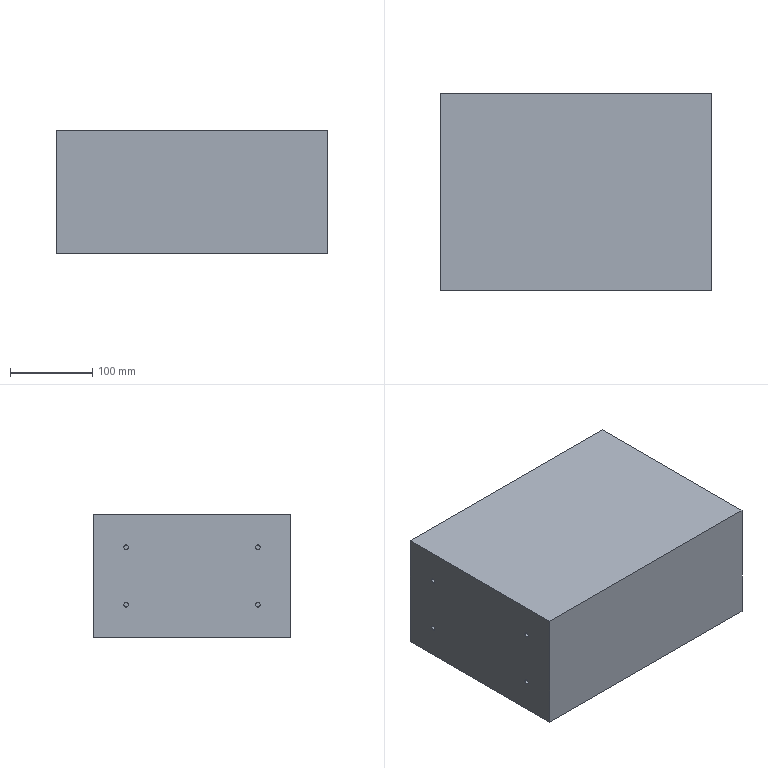Part | SolidWorks | features Cut 2, Extrusion 1 | 1 solid | 24 faces | box 330 x 240 x 150 mm | volume 11869232 mm3 | cylinder 12 | plane 12 | commonest cylinder face diameters 5.5 x8 25 x4
STEP:
#1=CARTESIAN_POINT('',(-155.,-77.25,40.));
#2=VERTEX_POINT('',#1);
#3=CARTESIAN_POINT('',(-155.,-82.75,40.));
#4=VERTEX_POINT('',#3);
#5=CARTESIAN_POINT('',(-155.,-80.,40.));
#6=DIRECTION('',(-1.,0.,0.));
#7=DIRECTION('',(0.,-1.,0.));
#8=AXIS2_PLACEMENT_3D('',#5,#6,#7);
#9=CIRCLE('',#8,2.75);
#10=EDGE_CURVE('',#2,#4,#9,.T.);
#11=ORIENTED_EDGE('',*,*,#10,.F.);
#12=CARTESIAN_POINT('',(-165.,-77.25,40.));
#13=VERTEX_POINT('',#12);
#14=CARTESIAN_POINT('',(-155.,-77.25,40.));
#15=DIRECTION('',(-1.,0.,0.));
#16=VECTOR('',#15,1000.);
#17=LINE('',#14,#16);
#18=EDGE_CURVE('',#2,#13,#17,.T.);
#19=ORIENTED_EDGE('',*,*,#18,.T.);
#20=CARTESIAN_POINT('',(-165.,-82.75,40.));
#21=VERTEX_POINT('',#20);
#22=CARTESIAN_POINT('',(-165.,-80.,40.));
#23=DIRECTION('',(-1.,0.,0.));
#24=DIRECTION('',(0.,-1.,0.));
#25=AXIS2_PLACEMENT_3D('',#22,#23,#24);
#26=CIRCLE('',#25,2.75);
#27=EDGE_CURVE('',#13,#21,#26,.T.);
#28=ORIENTED_EDGE('',*,*,#27,.T.);
#29=CARTESIAN_POINT('',(-155.,-82.75,40.));
#30=DIRECTION('',(-1.,0.,0.));
#31=VECTOR('',#30,1000.);
#32=LINE('',#29,#31);
#33=EDGE_CURVE('',#4,#21,#32,.T.);
#34=ORIENTED_EDGE('',*,*,#33,.F.);
#35=EDGE_LOOP('',(#11,#19,#28,#34));
#36=FACE_OUTER_BOUND('',#35,.T.);
#37=CARTESIAN_POINT('',(-155.,-80.,40.));
#38=DIRECTION('',(-1.,0.,0.));
#39=DIRECTION('',(0.,-1.,0.));
#40=AXIS2_PLACEMENT_3D('',#37,#38,#39);
#41=CYLINDRICAL_SURFACE('',#40,2.75);
#42=ADVANCED_FACE('',(#36),#41,.F.);
#43=CARTESIAN_POINT('',(-155.,-77.25,110.));
#44=VERTEX_POINT('',#43);
#45=CARTESIAN_POINT('',(-155.,-82.75,110.));
#46=VERTEX_POINT('',#45);
#47=CARTESIAN_POINT('',(-155.,-80.,110.));
#48=DIRECTION('',(-1.,0.,0.));
#49=DIRECTION('',(0.,-1.,0.));
#50=AXIS2_PLACEMENT_3D('',#47,#48,#49);
#51=CIRCLE('',#50,2.75);
#52=EDGE_CURVE('',#44,#46,#51,.T.);
#53=ORIENTED_EDGE('',*,*,#52,.F.);
#54=CARTESIAN_POINT('',(-165.,-77.25,110.));
#55=VERTEX_POINT('',#54);
#56=CARTESIAN_POINT('',(-155.,-77.25,110.));
#57=DIRECTION('',(-1.,0.,0.));
#58=VECTOR('',#57,1000.);
#59=LINE('',#56,#58);
#60=EDGE_CURVE('',#44,#55,#59,.T.);
#61=ORIENTED_EDGE('',*,*,#60,.T.);
#62=CARTESIAN_POINT('',(-165.,-82.75,110.));
#63=VERTEX_POINT('',#62);
#64=CARTESIAN_POINT('',(-165.,-80.,110.));
#65=DIRECTION('',(-1.,0.,0.));
#66=DIRECTION('',(0.,-1.,0.));
#67=AXIS2_PLACEMENT_3D('',#64,#65,#66);
#68=CIRCLE('',#67,2.75);
#69=EDGE_CURVE('',#55,#63,#68,.T.);
#70=ORIENTED_EDGE('',*,*,#69,.T.);
#71=CARTESIAN_POINT('',(-155.,-82.75,110.));
#72=DIRECTION('',(-1.,0.,0.));
#73=VECTOR('',#72,1000.);
#74=LINE('',#71,#73);
#75=EDGE_CURVE('',#46,#63,#74,.T.);
#76=ORIENTED_EDGE('',*,*,#75,.F.);
#77=EDGE_LOOP('',(#53,#61,#70,#76));
#78=FACE_OUTER_BOUND('',#77,.T.);
#79=CARTESIAN_POINT('',(-155.,-80.,110.));
#80=DIRECTION('',(-1.,0.,0.));
#81=DIRECTION('',(0.,-1.,0.));
#82=AXIS2_PLACEMENT_3D('',#79,#80,#81);
#83=CYLINDRICAL_SURFACE('',#82,2.75);
#84=ADVANCED_FACE('',(#78),#83,.F.);
#85=CARTESIAN_POINT('',(-155.,82.75,110.));
#86=VERTEX_POINT('',#85);
#87=CARTESIAN_POINT('',(-155.,77.25,110.));
#88=VERTEX_POINT('',#87);
#89=CARTESIAN_POINT('',(-155.,80.,110.));
#90=DIRECTION('',(-1.,0.,0.));
#91=DIRECTION('',(0.,-1.,0.));
#92=AXIS2_PLACEMENT_3D('',#89,#90,#91);
#93=CIRCLE('',#92,2.75);
#94=EDGE_CURVE('',#86,#88,#93,.T.);
#95=ORIENTED_EDGE('',*,*,#94,.F.);
#96=CARTESIAN_POINT('',(-165.,82.75,110.));
#97=VERTEX_POINT('',#96);
#98=CARTESIAN_POINT('',(-155.,82.75,110.));
#99=DIRECTION('',(-1.,0.,0.));
#100=VECTOR('',#99,1000.);
#101=LINE('',#98,#100);
#102=EDGE_CURVE('',#86,#97,#101,.T.);
#103=ORIENTED_EDGE('',*,*,#102,.T.);
#104=CARTESIAN_POINT('',(-165.,77.25,110.));
#105=VERTEX_POINT('',#104);
#106=CARTESIAN_POINT('',(-165.,80.,110.));
#107=DIRECTION('',(-1.,0.,0.));
#108=DIRECTION('',(0.,-1.,0.));
#109=AXIS2_PLACEMENT_3D('',#106,#107,#108);
#110=CIRCLE('',#109,2.75);
#111=EDGE_CURVE('',#97,#105,#110,.T.);
#112=ORIENTED_EDGE('',*,*,#111,.T.);
#113=CARTESIAN_POINT('',(-155.,77.25,110.));
#114=DIRECTION('',(-1.,0.,0.));
#115=VECTOR('',#114,1000.);
#116=LINE('',#113,#115);
#117=EDGE_CURVE('',#88,#105,#116,.T.);
#118=ORIENTED_EDGE('',*,*,#117,.F.);
#119=EDGE_LOOP('',(#95,#103,#112,#118));
#120=FACE_OUTER_BOUND('',#119,.T.);
#121=CARTESIAN_POINT('',(-155.,80.,110.));
#122=DIRECTION('',(-1.,0.,0.));
#123=DIRECTION('',(0.,-1.,0.));
#124=AXIS2_PLACEMENT_3D('',#121,#122,#123);
#125=CYLINDRICAL_SURFACE('',#124,2.75);
#126=ADVANCED_FACE('',(#120),#125,.F.);
#127=CARTESIAN_POINT('',(-155.,82.75,40.));
#128=VERTEX_POINT('',#127);
#129=CARTESIAN_POINT('',(-155.,77.25,40.));
#130=VERTEX_POINT('',#129);
#131=CARTESIAN_POINT('',(-155.,80.,40.));
#132=DIRECTION('',(-1.,0.,0.));
#133=DIRECTION('',(0.,-1.,0.));
#134=AXIS2_PLACEMENT_3D('',#131,#132,#133);
#135=CIRCLE('',#134,2.75);
#136=EDGE_CURVE('',#128,#130,#135,.T.);
#137=ORIENTED_EDGE('',*,*,#136,.F.);
#138=CARTESIAN_POINT('',(-165.,82.75,40.));
#139=VERTEX_POINT('',#138);
#140=CARTESIAN_POINT('',(-155.,82.75,40.));
#141=DIRECTION('',(-1.,0.,0.));
#142=VECTOR('',#141,1000.);
#143=LINE('',#140,#142);
#144=EDGE_CURVE('',#128,#139,#143,.T.);
#145=ORIENTED_EDGE('',*,*,#144,.T.);
#146=CARTESIAN_POINT('',(-165.,77.25,40.));
#147=VERTEX_POINT('',#146);
#148=CARTESIAN_POINT('',(-165.,80.,40.));
#149=DIRECTION('',(-1.,0.,0.));
#150=DIRECTION('',(0.,-1.,0.));
#151=AXIS2_PLACEMENT_3D('',#148,#149,#150);
#152=CIRCLE('',#151,2.75);
#153=EDGE_CURVE('',#139,#147,#152,.T.);
#154=ORIENTED_EDGE('',*,*,#153,.T.);
#155=CARTESIAN_POINT('',(-155.,77.25,40.));
#156=DIRECTION('',(-1.,0.,0.));
#157=VECTOR('',#156,1000.);
#158=LINE('',#155,#157);
#159=EDGE_CURVE('',#130,#147,#158,.T.);
#160=ORIENTED_EDGE('',*,*,#159,.F.);
#161=EDGE_LOOP('',(#137,#145,#154,#160));
#162=FACE_OUTER_BOUND('',#161,.T.);
#163=CARTESIAN_POINT('',(-155.,80.,40.));
#164=DIRECTION('',(-1.,0.,0.));
#165=DIRECTION('',(0.,-1.,0.));
#166=AXIS2_PLACEMENT_3D('',#163,#164,#165);
#167=CYLINDRICAL_SURFACE('',#166,2.75);
#168=ADVANCED_FACE('',(#162),#167,.F.);
#169=CARTESIAN_POINT('',(155.,-72.5,75.));
#170=VERTEX_POINT('',#169);
#171=CARTESIAN_POINT('',(155.,-47.5,75.));
#172=VERTEX_POINT('',#171);
#173=CARTESIAN_POINT('',(155.,-60.,75.));
#174=DIRECTION('',(1.,0.,0.));
#175=DIRECTION('',(0.,1.,0.));
#176=AXIS2_PLACEMENT_3D('',#173,#174,#175);
#177=CIRCLE('',#176,12.5);
#178=EDGE_CURVE('',#170,#172,#177,.T.);
#179=ORIENTED_EDGE('',*,*,#178,.F.);
#180=CARTESIAN_POINT('',(165.,-72.5,75.));
#181=VERTEX_POINT('',#180);
#182=CARTESIAN_POINT('',(155.,-72.5,75.));
#183=DIRECTION('',(1.,0.,0.));
#184=VECTOR('',#183,1000.);
#185=LINE('',#182,#184);
#186=EDGE_CURVE('',#170,#181,#185,.T.);
#187=ORIENTED_EDGE('',*,*,#186,.T.);
#188=CARTESIAN_POINT('',(165.,-47.5,75.));
#189=VERTEX_POINT('',#188);
#190=CARTESIAN_POINT('',(165.,-60.,75.));
#191=DIRECTION('',(1.,0.,0.));
#192=DIRECTION('',(0.,1.,0.));
#193=AXIS2_PLACEMENT_3D('',#190,#191,#192);
#194=CIRCLE('',#193,12.5);
#195=EDGE_CURVE('',#181,#189,#194,.T.);
#196=ORIENTED_EDGE('',*,*,#195,.T.);
#197=CARTESIAN_POINT('',(155.,-47.5,75.));
#198=DIRECTION('',(1.,0.,0.));
#199=VECTOR('',#198,1000.);
#200=LINE('',#197,#199);
#201=EDGE_CURVE('',#172,#189,#200,.T.);
#202=ORIENTED_EDGE('',*,*,#201,.F.);
#203=EDGE_LOOP('',(#179,#187,#196,#202));
#204=FACE_OUTER_BOUND('',#203,.T.);
#205=CARTESIAN_POINT('',(155.,-60.,75.));
#206=DIRECTION('',(1.,0.,0.));
#207=DIRECTION('',(0.,1.,0.));
#208=AXIS2_PLACEMENT_3D('',#205,#206,#207);
#209=CYLINDRICAL_SURFACE('',#208,12.5);
#210=ADVANCED_FACE('',(#204),#209,.F.);
#211=CARTESIAN_POINT('',(155.,47.5,75.));
#212=VERTEX_POINT('',#211);
#213=CARTESIAN_POINT('',(155.,72.5,75.));
#214=VERTEX_POINT('',#213);
#215=CARTESIAN_POINT('',(155.,60.,75.));
#216=DIRECTION('',(1.,0.,0.));
#217=DIRECTION('',(0.,1.,0.));
#218=AXIS2_PLACEMENT_3D('',#215,#216,#217);
#219=CIRCLE('',#218,12.5);
#220=EDGE_CURVE('',#212,#214,#219,.T.);
#221=ORIENTED_EDGE('',*,*,#220,.F.);
#222=CARTESIAN_POINT('',(165.,47.5,75.));
#223=VERTEX_POINT('',#222);
#224=CARTESIAN_POINT('',(155.,47.5,75.));
#225=DIRECTION('',(1.,0.,0.));
#226=VECTOR('',#225,1000.);
#227=LINE('',#224,#226);
#228=EDGE_CURVE('',#212,#223,#227,.T.);
#229=ORIENTED_EDGE('',*,*,#228,.T.);
#230=CARTESIAN_POINT('',(165.,72.5,75.));
#231=VERTEX_POINT('',#230);
#232=CARTESIAN_POINT('',(165.,60.,75.));
#233=DIRECTION('',(1.,0.,0.));
#234=DIRECTION('',(0.,1.,0.));
#235=AXIS2_PLACEMENT_3D('',#232,#233,#234);
#236=CIRCLE('',#235,12.5);
#237=EDGE_CURVE('',#223,#231,#236,.T.);
#238=ORIENTED_EDGE('',*,*,#237,.T.);
#239=CARTESIAN_POINT('',(155.,72.5,75.));
#240=DIRECTION('',(1.,0.,0.));
#241=VECTOR('',#240,1000.);
#242=LINE('',#239,#241);
#243=EDGE_CURVE('',#214,#231,#242,.T.);
#244=ORIENTED_EDGE('',*,*,#243,.F.);
#245=EDGE_LOOP('',(#221,#229,#238,#244));
#246=FACE_OUTER_BOUND('',#245,.T.);
#247=CARTESIAN_POINT('',(155.,60.,75.));
#248=DIRECTION('',(1.,0.,0.));
#249=DIRECTION('',(0.,1.,0.));
#250=AXIS2_PLACEMENT_3D('',#247,#248,#249);
#251=CYLINDRICAL_SURFACE('',#250,12.5);
#252=ADVANCED_FACE('',(#246),#251,.F.);
#253=CARTESIAN_POINT('',(165.,-60.,75.));
#254=DIRECTION('',(1.,0.,0.));
#255=DIRECTION('',(0.,1.,0.));
#256=AXIS2_PLACEMENT_3D('',#253,#254,#255);
#257=CIRCLE('',#256,12.5);
#258=EDGE_CURVE('',#189,#181,#257,.T.);
#259=ORIENTED_EDGE('',*,*,#258,.F.);
#260=ORIENTED_EDGE('',*,*,#195,.F.);
#261=EDGE_LOOP('',(#259,#260));
#262=FACE_BOUND('',#261,.T.);
#263=CARTESIAN_POINT('',(165.,60.,75.));
#264=DIRECTION('',(1.,0.,0.));
#265=DIRECTION('',(0.,1.,0.));
#266=AXIS2_PLACEMENT_3D('',#263,#264,#265);
#267=CIRCLE('',#266,12.5);
#268=EDGE_CURVE('',#231,#223,#267,.T.);
#269=ORIENTED_EDGE('',*,*,#268,.F.);
#270=ORIENTED_EDGE('',*,*,#237,.F.);
#271=EDGE_LOOP('',(#269,#270));
#272=FACE_BOUND('',#271,.T.);
#273=CARTESIAN_POINT('',(165.,-120.,0.));
#274=VERTEX_POINT('',#273);
#275=CARTESIAN_POINT('',(165.,120.,0.));
#276=VERTEX_POINT('',#275);
#277=CARTESIAN_POINT('',(165.,120.,0.));
#278=DIRECTION('',(0.,1.,0.));
#279=VECTOR('',#278,1000.);
#280=LINE('',#277,#279);
#281=EDGE_CURVE('',#274,#276,#280,.T.);
#282=ORIENTED_EDGE('',*,*,#281,.T.);
#283=CARTESIAN_POINT('',(165.,120.,150.));
#284=VERTEX_POINT('',#283);
#285=CARTESIAN_POINT('',(165.,120.,150.));
#286=DIRECTION('',(0.,0.,-1.));
#287=VECTOR('',#286,1000.);
#288=LINE('',#285,#287);
#289=EDGE_CURVE('',#284,#276,#288,.T.);
#290=ORIENTED_EDGE('',*,*,#289,.F.);
#291=CARTESIAN_POINT('',(165.,-120.,150.));
#292=VERTEX_POINT('',#291);
#293=CARTESIAN_POINT('',(165.,120.,150.));
#294=DIRECTION('',(0.,1.,0.));
#295=VECTOR('',#294,1000.);
#296=LINE('',#293,#295);
#297=EDGE_CURVE('',#292,#284,#296,.T.);
#298=ORIENTED_EDGE('',*,*,#297,.F.);
#299=CARTESIAN_POINT('',(165.,-120.,150.));
#300=DIRECTION('',(0.,0.,-1.));
#301=VECTOR('',#300,1000.);
#302=LINE('',#299,#301);
#303=EDGE_CURVE('',#292,#274,#302,.T.);
#304=ORIENTED_EDGE('',*,*,#303,.T.);
#305=EDGE_LOOP('',(#282,#290,#298,#304));
#306=FACE_OUTER_BOUND('',#305,.T.);
#307=CARTESIAN_POINT('',(165.,120.,150.));
#308=DIRECTION('',(-1.,0.,0.));
#309=DIRECTION('',(0.,-1.,0.));
#310=AXIS2_PLACEMENT_3D('',#307,#308,#309);
#311=PLANE('',#310);
#312=ADVANCED_FACE('',(#262,#272,#306),#311,.F.);
#313=CARTESIAN_POINT('',(-165.,120.,0.));
#314=VERTEX_POINT('',#313);
#315=CARTESIAN_POINT('',(-165.,120.,0.));
#316=DIRECTION('',(-1.,0.,0.));
#317=VECTOR('',#316,1000.);
#318=LINE('',#315,#317);
#319=EDGE_CURVE('',#276,#314,#318,.T.);
#320=ORIENTED_EDGE('',*,*,#319,.T.);
#321=CARTESIAN_POINT('',(-165.,120.,150.));
#322=VERTEX_POINT('',#321);
#323=CARTESIAN_POINT('',(-165.,120.,150.));
#324=DIRECTION('',(0.,0.,-1.));
#325=VECTOR('',#324,1000.);
#326=LINE('',#323,#325);
#327=EDGE_CURVE('',#322,#314,#326,.T.);
#328=ORIENTED_EDGE('',*,*,#327,.F.);
#329=CARTESIAN_POINT('',(-165.,120.,150.));
#330=DIRECTION('',(-1.,0.,0.));
#331=VECTOR('',#330,1000.);
#332=LINE('',#329,#331);
#333=EDGE_CURVE('',#284,#322,#332,.T.);
#334=ORIENTED_EDGE('',*,*,#333,.F.);
#335=ORIENTED_EDGE('',*,*,#289,.T.);
#336=EDGE_LOOP('',(#320,#328,#334,#335));
#337=FACE_OUTER_BOUND('',#336,.T.);
#338=CARTESIAN_POINT('',(-165.,120.,150.));
#339=DIRECTION('',(0.,-1.,0.));
#340=DIRECTION('',(0.,0.,-1.));
#341=AXIS2_PLACEMENT_3D('',#338,#339,#340);
#342=PLANE('',#341);
#343=ADVANCED_FACE('',(#337),#342,.F.);
#344=CARTESIAN_POINT('',(-165.,-80.,40.));
#345=DIRECTION('',(-1.,0.,0.));
#346=DIRECTION('',(0.,-1.,0.));
#347=AXIS2_PLACEMENT_3D('',#344,#345,#346);
#348=CIRCLE('',#347,2.75);
#349=EDGE_CURVE('',#21,#13,#348,.T.);
#350=ORIENTED_EDGE('',*,*,#349,.F.);
#351=ORIENTED_EDGE('',*,*,#27,.F.);
#352=EDGE_LOOP('',(#350,#351));
#353=FACE_BOUND('',#352,.T.);
#354=CARTESIAN_POINT('',(-165.,-80.,110.));
#355=DIRECTION('',(-1.,0.,0.));
#356=DIRECTION('',(0.,-1.,0.));
#357=AXIS2_PLACEMENT_3D('',#354,#355,#356);
#358=CIRCLE('',#357,2.75);
#359=EDGE_CURVE('',#63,#55,#358,.T.);
#360=ORIENTED_EDGE('',*,*,#359,.F.);
#361=ORIENTED_EDGE('',*,*,#69,.F.);
#362=EDGE_LOOP('',(#360,#361));
#363=FACE_BOUND('',#362,.T.);
#364=CARTESIAN_POINT('',(-165.,80.,110.));
#365=DIRECTION('',(-1.,0.,0.));
#366=DIRECTION('',(0.,-1.,0.));
#367=AXIS2_PLACEMENT_3D('',#364,#365,#366);
#368=CIRCLE('',#367,2.75);
#369=EDGE_CURVE('',#105,#97,#368,.T.);
#370=ORIENTED_EDGE('',*,*,#369,.F.);
#371=ORIENTED_EDGE('',*,*,#111,.F.);
#372=EDGE_LOOP('',(#370,#371));
#373=FACE_BOUND('',#372,.T.);
#374=CARTESIAN_POINT('',(-165.,80.,40.));
#375=DIRECTION('',(-1.,0.,0.));
#376=DIRECTION('',(0.,-1.,0.));
#377=AXIS2_PLACEMENT_3D('',#374,#375,#376);
#378=CIRCLE('',#377,2.75);
#379=EDGE_CURVE('',#147,#139,#378,.T.);
#380=ORIENTED_EDGE('',*,*,#379,.F.);
#381=ORIENTED_EDGE('',*,*,#153,.F.);
#382=EDGE_LOOP('',(#380,#381));
#383=FACE_BOUND('',#382,.T.);
#384=CARTESIAN_POINT('',(-165.,-120.,0.));
#385=VERTEX_POINT('',#384);
#386=CARTESIAN_POINT('',(-165.,120.,0.));
#387=DIRECTION('',(0.,-1.,0.));
#388=VECTOR('',#387,1000.);
#389=LINE('',#386,#388);
#390=EDGE_CURVE('',#314,#385,#389,.T.);
#391=ORIENTED_EDGE('',*,*,#390,.T.);
#392=CARTESIAN_POINT('',(-165.,-120.,150.));
#393=VERTEX_POINT('',#392);
#394=CARTESIAN_POINT('',(-165.,-120.,150.));
#395=DIRECTION('',(0.,0.,-1.));
#396=VECTOR('',#395,1000.);
#397=LINE('',#394,#396);
#398=EDGE_CURVE('',#393,#385,#397,.T.);
#399=ORIENTED_EDGE('',*,*,#398,.F.);
#400=CARTESIAN_POINT('',(-165.,120.,150.));
#401=DIRECTION('',(0.,-1.,0.));
#402=VECTOR('',#401,1000.);
#403=LINE('',#400,#402);
#404=EDGE_CURVE('',#322,#393,#403,.T.);
#405=ORIENTED_EDGE('',*,*,#404,.F.);
#406=ORIENTED_EDGE('',*,*,#327,.T.);
#407=EDGE_LOOP('',(#391,#399,#405,#406));
#408=FACE_OUTER_BOUND('',#407,.T.);
#409=CARTESIAN_POINT('',(-165.,120.,150.));
#410=DIRECTION('',(1.,0.,0.));
#411=DIRECTION('',(0.,0.,-1.));
#412=AXIS2_PLACEMENT_3D('',#409,#410,#411);
#413=PLANE('',#412);
#414=ADVANCED_FACE('',(#353,#363,#373,#383,#408),#413,.F.);
#415=CARTESIAN_POINT('',(-165.,-120.,0.));
#416=DIRECTION('',(1.,0.,0.));
#417=VECTOR('',#416,1000.);
#418=LINE('',#415,#417);
#419=EDGE_CURVE('',#385,#274,#418,.T.);
#420=ORIENTED_EDGE('',*,*,#419,.T.);
#421=ORIENTED_EDGE('',*,*,#303,.F.);
#422=CARTESIAN_POINT('',(-165.,-120.,150.));
#423=DIRECTION('',(1.,0.,0.));
#424=VECTOR('',#423,1000.);
#425=LINE('',#422,#424);
#426=EDGE_CURVE('',#393,#292,#425,.T.);
#427=ORIENTED_EDGE('',*,*,#426,.F.);
#428=ORIENTED_EDGE('',*,*,#398,.T.);
#429=EDGE_LOOP('',(#420,#421,#427,#428));
#430=FACE_OUTER_BOUND('',#429,.T.);
#431=CARTESIAN_POINT('',(-165.,-120.,150.));
#432=DIRECTION('',(0.,1.,0.));
#433=DIRECTION('',(0.,0.,1.));
#434=AXIS2_PLACEMENT_3D('',#431,#432,#433);
#435=PLANE('',#434);
#436=ADVANCED_FACE('',(#430),#435,.F.);
#437=ORIENTED_EDGE('',*,*,#297,.T.);
#438=ORIENTED_EDGE('',*,*,#333,.T.);
#439=ORIENTED_EDGE('',*,*,#404,.T.);
#440=ORIENTED_EDGE('',*,*,#426,.T.);
#441=EDGE_LOOP('',(#437,#438,#439,#440));
#442=FACE_OUTER_BOUND('',#441,.T.);
#443=CARTESIAN_POINT('',(0.,0.,150.));
#444=DIRECTION('',(0.,0.,1.));
#445=DIRECTION('',(1.,0.,0.));
#446=AXIS2_PLACEMENT_3D('',#443,#444,#445);
#447=PLANE('',#446);
#448=ADVANCED_FACE('',(#442),#447,.T.);
#449=ORIENTED_EDGE('',*,*,#281,.F.);
#450=ORIENTED_EDGE('',*,*,#419,.F.);
#451=ORIENTED_EDGE('',*,*,#390,.F.);
#452=ORIENTED_EDGE('',*,*,#319,.F.);
#453=EDGE_LOOP('',(#449,#450,#451,#452));
#454=FACE_OUTER_BOUND('',#453,.T.);
#455=CARTESIAN_POINT('',(0.,0.,0.));
#456=DIRECTION('',(0.,0.,1.));
#457=DIRECTION('',(1.,0.,0.));
#458=AXIS2_PLACEMENT_3D('',#455,#456,#457);
#459=PLANE('',#458);
#460=ADVANCED_FACE('',(#454),#459,.F.);
#461=ORIENTED_EDGE('',*,*,#228,.F.);
#462=CARTESIAN_POINT('',(155.,60.,75.));
#463=DIRECTION('',(1.,0.,0.));
#464=DIRECTION('',(0.,1.,0.));
#465=AXIS2_PLACEMENT_3D('',#462,#463,#464);
#466=CIRCLE('',#465,12.5);
#467=EDGE_CURVE('',#214,#212,#466,.T.);
#468=ORIENTED_EDGE('',*,*,#467,.F.);
#469=ORIENTED_EDGE('',*,*,#243,.T.);
#470=ORIENTED_EDGE('',*,*,#268,.T.);
#471=EDGE_LOOP('',(#461,#468,#469,#470));
#472=FACE_OUTER_BOUND('',#471,.T.);
#473=CARTESIAN_POINT('',(155.,60.,75.));
#474=DIRECTION('',(1.,0.,0.));
#475=DIRECTION('',(0.,1.,0.));
#476=AXIS2_PLACEMENT_3D('',#473,#474,#475);
#477=CYLINDRICAL_SURFACE('',#476,12.5);
#478=ADVANCED_FACE('',(#472),#477,.F.);
#479=ORIENTED_EDGE('',*,*,#467,.T.);
#480=ORIENTED_EDGE('',*,*,#220,.T.);
#481=EDGE_LOOP('',(#479,#480));
#482=FACE_OUTER_BOUND('',#481,.T.);
#483=CARTESIAN_POINT('',(155.,60.,75.));
#484=DIRECTION('',(1.,0.,0.));
#485=DIRECTION('',(0.,1.,0.));
#486=AXIS2_PLACEMENT_3D('',#483,#484,#485);
#487=PLANE('',#486);
#488=ADVANCED_FACE('',(#482),#487,.T.);
#489=ORIENTED_EDGE('',*,*,#186,.F.);
#490=CARTESIAN_POINT('',(155.,-60.,75.));
#491=DIRECTION('',(1.,0.,0.));
#492=DIRECTION('',(0.,1.,0.));
#493=AXIS2_PLACEMENT_3D('',#490,#491,#492);
#494=CIRCLE('',#493,12.5);
#495=EDGE_CURVE('',#172,#170,#494,.T.);
#496=ORIENTED_EDGE('',*,*,#495,.F.);
#497=ORIENTED_EDGE('',*,*,#201,.T.);
#498=ORIENTED_EDGE('',*,*,#258,.T.);
#499=EDGE_LOOP('',(#489,#496,#497,#498));
#500=FACE_OUTER_BOUND('',#499,.T.);
#501=CARTESIAN_POINT('',(155.,-60.,75.));
#502=DIRECTION('',(1.,0.,0.));
#503=DIRECTION('',(0.,1.,0.));
#504=AXIS2_PLACEMENT_3D('',#501,#502,#503);
#505=CYLINDRICAL_SURFACE('',#504,12.5);
#506=ADVANCED_FACE('',(#500),#505,.F.);
#507=ORIENTED_EDGE('',*,*,#495,.T.);
#508=ORIENTED_EDGE('',*,*,#178,.T.);
#509=EDGE_LOOP('',(#507,#508));
#510=FACE_OUTER_BOUND('',#509,.T.);
#511=CARTESIAN_POINT('',(155.,-60.,75.));
#512=DIRECTION('',(1.,0.,0.));
#513=DIRECTION('',(0.,1.,0.));
#514=AXIS2_PLACEMENT_3D('',#511,#512,#513);
#515=PLANE('',#514);
#516=ADVANCED_FACE('',(#510),#515,.T.);
#517=ORIENTED_EDGE('',*,*,#144,.F.);
#518=CARTESIAN_POINT('',(-155.,80.,40.));
#519=DIRECTION('',(-1.,0.,0.));
#520=DIRECTION('',(0.,-1.,0.));
#521=AXIS2_PLACEMENT_3D('',#518,#519,#520);
#522=CIRCLE('',#521,2.75);
#523=EDGE_CURVE('',#130,#128,#522,.T.);
#524=ORIENTED_EDGE('',*,*,#523,.F.);
#525=ORIENTED_EDGE('',*,*,#159,.T.);
#526=ORIENTED_EDGE('',*,*,#379,.T.);
#527=EDGE_LOOP('',(#517,#524,#525,#526));
#528=FACE_OUTER_BOUND('',#527,.T.);
#529=CARTESIAN_POINT('',(-155.,80.,40.));
#530=DIRECTION('',(-1.,0.,0.));
#531=DIRECTION('',(0.,-1.,0.));
#532=AXIS2_PLACEMENT_3D('',#529,#530,#531);
#533=CYLINDRICAL_SURFACE('',#532,2.75);
#534=ADVANCED_FACE('',(#528),#533,.F.);
#535=ORIENTED_EDGE('',*,*,#523,.T.);
#536=ORIENTED_EDGE('',*,*,#136,.T.);
#537=EDGE_LOOP('',(#535,#536));
#538=FACE_OUTER_BOUND('',#537,.T.);
#539=CARTESIAN_POINT('',(-155.,80.,40.));
#540=DIRECTION('',(-1.,0.,0.));
#541=DIRECTION('',(0.,-1.,0.));
#542=AXIS2_PLACEMENT_3D('',#539,#540,#541);
#543=PLANE('',#542);
#544=ADVANCED_FACE('',(#538),#543,.T.);
#545=ORIENTED_EDGE('',*,*,#102,.F.);
#546=CARTESIAN_POINT('',(-155.,80.,110.));
#547=DIRECTION('',(-1.,0.,0.));
#548=DIRECTION('',(0.,-1.,0.));
#549=AXIS2_PLACEMENT_3D('',#546,#547,#548);
#550=CIRCLE('',#549,2.75);
#551=EDGE_CURVE('',#88,#86,#550,.T.);
#552=ORIENTED_EDGE('',*,*,#551,.F.);
#553=ORIENTED_EDGE('',*,*,#117,.T.);
#554=ORIENTED_EDGE('',*,*,#369,.T.);
#555=EDGE_LOOP('',(#545,#552,#553,#554));
#556=FACE_OUTER_BOUND('',#555,.T.);
#557=CARTESIAN_POINT('',(-155.,80.,110.));
#558=DIRECTION('',(-1.,0.,0.));
#559=DIRECTION('',(0.,-1.,0.));
#560=AXIS2_PLACEMENT_3D('',#557,#558,#559);
#561=CYLINDRICAL_SURFACE('',#560,2.75);
#562=ADVANCED_FACE('',(#556),#561,.F.);
#563=ORIENTED_EDGE('',*,*,#551,.T.);
#564=ORIENTED_EDGE('',*,*,#94,.T.);
#565=EDGE_LOOP('',(#563,#564));
#566=FACE_OUTER_BOUND('',#565,.T.);
#567=CARTESIAN_POINT('',(-155.,80.,110.));
#568=DIRECTION('',(-1.,0.,0.));
#569=DIRECTION('',(0.,-1.,0.));
#570=AXIS2_PLACEMENT_3D('',#567,#568,#569);
#571=PLANE('',#570);
#572=ADVANCED_FACE('',(#566),#571,.T.);
#573=ORIENTED_EDGE('',*,*,#60,.F.);
#574=CARTESIAN_POINT('',(-155.,-80.,110.));
#575=DIRECTION('',(-1.,0.,0.));
#576=DIRECTION('',(0.,-1.,0.));
#577=AXIS2_PLACEMENT_3D('',#574,#575,#576);
#578=CIRCLE('',#577,2.75);
#579=EDGE_CURVE('',#46,#44,#578,.T.);
#580=ORIENTED_EDGE('',*,*,#579,.F.);
#581=ORIENTED_EDGE('',*,*,#75,.T.);
#582=ORIENTED_EDGE('',*,*,#359,.T.);
#583=EDGE_LOOP('',(#573,#580,#581,#582));
#584=FACE_OUTER_BOUND('',#583,.T.);
#585=CARTESIAN_POINT('',(-155.,-80.,110.));
#586=DIRECTION('',(-1.,0.,0.));
#587=DIRECTION('',(0.,-1.,0.));
#588=AXIS2_PLACEMENT_3D('',#585,#586,#587);
#589=CYLINDRICAL_SURFACE('',#588,2.75);
#590=ADVANCED_FACE('',(#584),#589,.F.);
#591=ORIENTED_EDGE('',*,*,#579,.T.);
#592=ORIENTED_EDGE('',*,*,#52,.T.);
#593=EDGE_LOOP('',(#591,#592));
#594=FACE_OUTER_BOUND('',#593,.T.);
#595=CARTESIAN_POINT('',(-155.,-80.,110.));
#596=DIRECTION('',(-1.,0.,0.));
#597=DIRECTION('',(0.,-1.,0.));
#598=AXIS2_PLACEMENT_3D('',#595,#596,#597);
#599=PLANE('',#598);
#600=ADVANCED_FACE('',(#594),#599,.T.);
#601=ORIENTED_EDGE('',*,*,#18,.F.);
#602=CARTESIAN_POINT('',(-155.,-80.,40.));
#603=DIRECTION('',(-1.,0.,0.));
#604=DIRECTION('',(0.,-1.,0.));
#605=AXIS2_PLACEMENT_3D('',#602,#603,#604);
#606=CIRCLE('',#605,2.75);
#607=EDGE_CURVE('',#4,#2,#606,.T.);
#608=ORIENTED_EDGE('',*,*,#607,.F.);
#609=ORIENTED_EDGE('',*,*,#33,.T.);
#610=ORIENTED_EDGE('',*,*,#349,.T.);
#611=EDGE_LOOP('',(#601,#608,#609,#610));
#612=FACE_OUTER_BOUND('',#611,.T.);
#613=CARTESIAN_POINT('',(-155.,-80.,40.));
#614=DIRECTION('',(-1.,0.,0.));
#615=DIRECTION('',(0.,-1.,0.));
#616=AXIS2_PLACEMENT_3D('',#613,#614,#615);
#617=CYLINDRICAL_SURFACE('',#616,2.75);
#618=ADVANCED_FACE('',(#612),#617,.F.);
#619=ORIENTED_EDGE('',*,*,#607,.T.);
#620=ORIENTED_EDGE('',*,*,#10,.T.);
#621=EDGE_LOOP('',(#619,#620));
#622=FACE_OUTER_BOUND('',#621,.T.);
#623=CARTESIAN_POINT('',(-155.,-80.,40.));
#624=DIRECTION('',(-1.,0.,0.));
#625=DIRECTION('',(0.,-1.,0.));
#626=AXIS2_PLACEMENT_3D('',#623,#624,#625);
#627=PLANE('',#626);
#628=ADVANCED_FACE('',(#622),#627,.T.);
#629=CLOSED_SHELL('',(#42,#84,#126,#168,#210,#252,#312,#343,#414,#436,#448,#460,#478,#488,#506,#516,#534,#544,#562,#572,#590,#600,#618,#628));
#630=MANIFOLD_SOLID_BREP('',#629);
#631=CARTESIAN_POINT('',(0.,0.,0.));
#632=DIRECTION('',(0.,0.,1.));
#633=DIRECTION('',(1.,0.,0.));
#634=AXIS2_PLACEMENT_3D('',#631,#632,#633);
#635=(LENGTH_UNIT()NAMED_UNIT(*)SI_UNIT(.MILLI.,.METRE.));
#636=UNCERTAINTY_MEASURE_WITH_UNIT(LENGTH_MEASURE(0.00001),#635,'','');
#637=(NAMED_UNIT(*)PLANE_ANGLE_UNIT()SI_UNIT($,.RADIAN.));
#638=(NAMED_UNIT(*)SI_UNIT($,.STERADIAN.)SOLID_ANGLE_UNIT());
#639=(GEOMETRIC_REPRESENTATION_CONTEXT(3)GLOBAL_UNCERTAINTY_ASSIGNED_CONTEXT((#636))GLOBAL_UNIT_ASSIGNED_CONTEXT((#635,#637,#638))REPRESENTATION_CONTEXT('',''));
#640=ADVANCED_BREP_SHAPE_REPRESENTATION('',(#630,#634),#639);